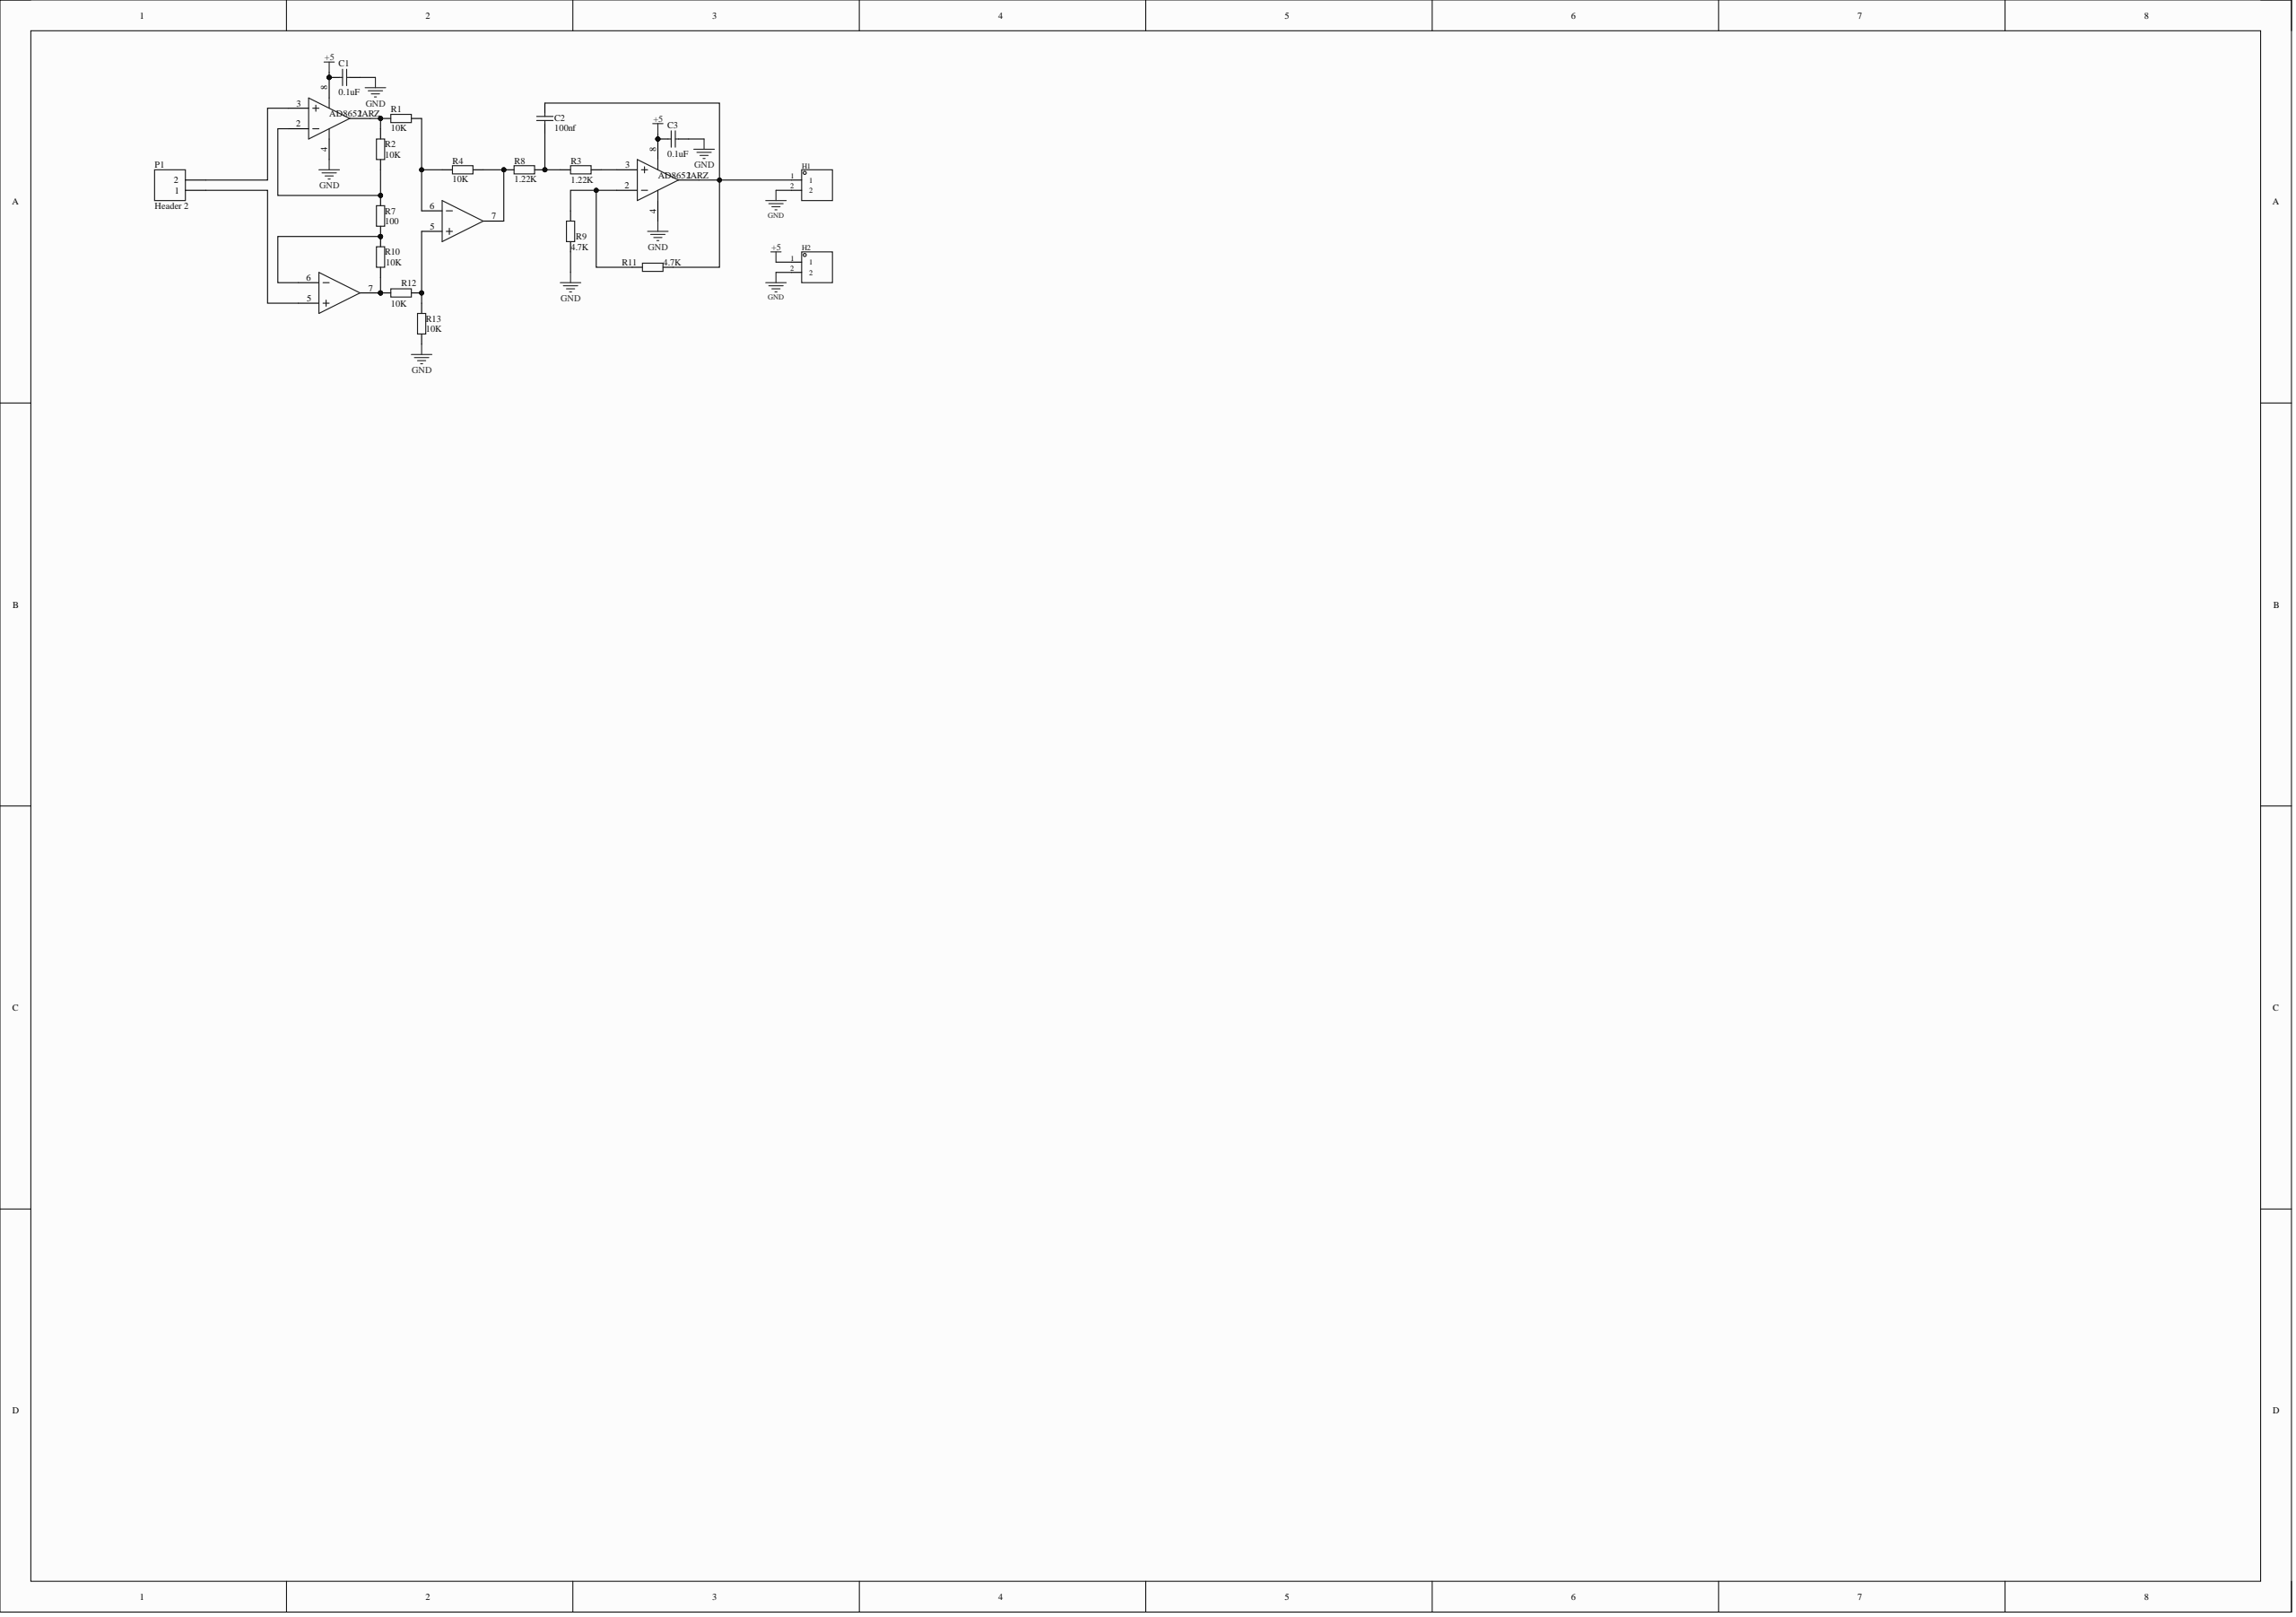Circuit board | Altium Designer | 19 parts | 15 nets
Bill of materials:
Comment,Description,Designator,Footprint,LibRef,Quantity
"Cap","Capacitor","C1, C2, C3","CAP-TH_L5.0-W2.5-P5.00-D1.0","Cap","3"
"","","H1, H2","HDR-TH_2P-P2.54-V-M-1","HDR-M_2.54_1x2P","2"
"Header 2","Header, 2-Pin","P1","HDR-TH_2P-P2.54-V-M-1","Header 2","1"
"10K","Resistor","R1, R2, R4, R10, R12, R13","R0603_SMD-CRCW060327R0FKEA","10K_1, 10K","6"
"1.22K","Resistor","R3, R8","R0603_SMD-CRCW060327R0FKEA","1.22K","2"
"100","Resistor","R7","R0603_SMD-CRCW060327R0FKEA","100","1"
"4.7K","Resistor","R9, R11","R0603_SMD-CRCW060327R0FKEA","4.7K, 4.7K_1","2"
"AD8652ARZ","","U1, U2","SOIC-8_L4.9-W3.9-P1.27-LS6.0-BL","AD8652ARZ","2"
Netlist (Protel format):
[
C1
CAP-TH_L5.0-W2.5-P5.00-D1.0
Cap



]
[
C2
CAP-TH_L5.0-W2.5-P5.00-D1.0
Cap



]
[
C3
CAP-TH_L5.0-W2.5-P5.00-D1.0
Cap



]
[
H1
HDR-TH_2P-P2.54-V-M-1




]
[
H2
HDR-TH_2P-P2.54-V-M-1




]
[
P1
HDR-TH_2P-P2.54-V-M-1
Header 2



]
[
R1
R0603_SMD-CRCW060327R0FKEA
10K



]
[
R2
R0603_SMD-CRCW060327R0FKEA
10K



]
[
R3
R0603_SMD-CRCW060327R0FKEA
1.22K



]
[
R4
R0603_SMD-CRCW060327R0FKEA
10K



]
[
R7
R0603_SMD-CRCW060327R0FKEA
100



]
[
R8
R0603_SMD-CRCW060327R0FKEA
1.22K



]
[
R9
R0603_SMD-CRCW060327R0FKEA
4.7K



]
[
R10
R0603_SMD-CRCW060327R0FKEA
10K



]
[
R11
R0603_SMD-CRCW060327R0FKEA
4.7K



]
[
R12
R0603_SMD-CRCW060327R0FKEA
10K



]
[
R13
R0603_SMD-CRCW060327R0FKEA
10K



]
[
U1
SOIC-8_L4.9-W3.9-P1.27-LS6.0-BL
AD8652ARZ



]
[
U2
SOIC-8_L4.9-W3.9-P1.27-LS6.0-BL
AD8652ARZ



]
(
NetR12_1
R12-1
R13-1
U2-5
)
(
NetR10_1
R10-1
R12-2
U1-7
)
(
NetR9_2
R9-2
R11-1
U2-2
)
(
NetR7_1
R7-1
R10-2
U1-6
)
(
NetR4_1
R4-1
R8-1
U2-7
)
(
NetR3_2
R3-2
U2-3
)
(
NetR2_1
R2-1
R7-2
U1-2
)
(
NetR1_2
R1-2
R2-2
U1-1
)
(
NetR1_1
R1-1
R4-2
U2-6
)
(
NetP1_2
P1-2
U1-3
)
(
NetP1_1
P1-1
U1-5
)
(
NetC2_2
C2-2
R3-1
R8-2
)
(
NetC2_1
C2-1
H1-1
R11-2
U2-1
)
(
GND
C1-2
C3-2
H1-2
H2-2
R9-1
R13-2
U1-4
U2-4
)
(
+5
C1-1
C3-1
H2-1
U1-8
U2-8
)